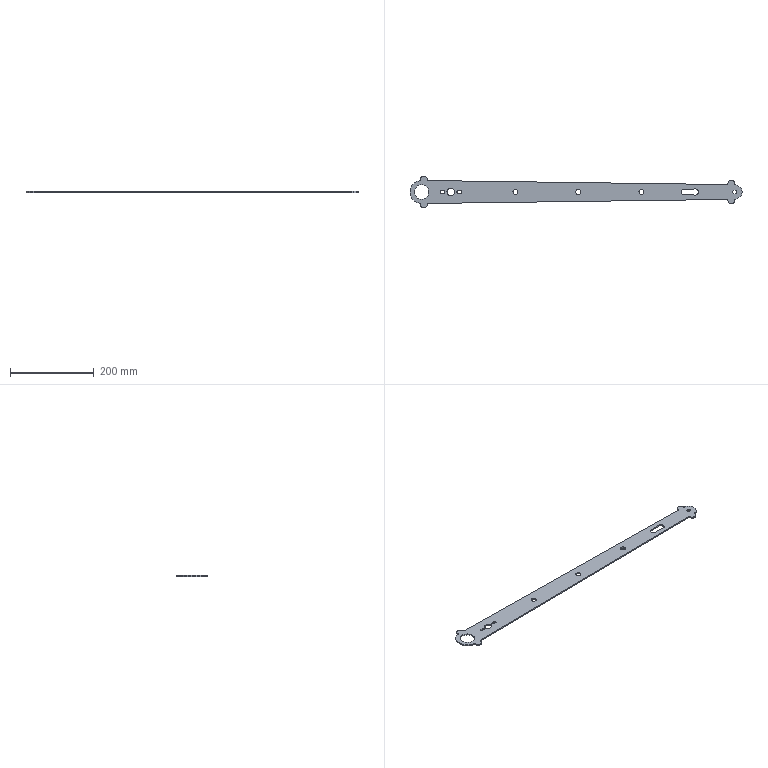Part | STEP file | Belt guard plate QY-1-32 | 1 solid | 56 faces | box 791 x 76.328 x 3 mm | volume 100631 mm3 | cylinder 42 | plane 14 | commonest cylinder face diameters 6 x10 16 x10 6.5 x6 12 x6 35 x4 9 x3